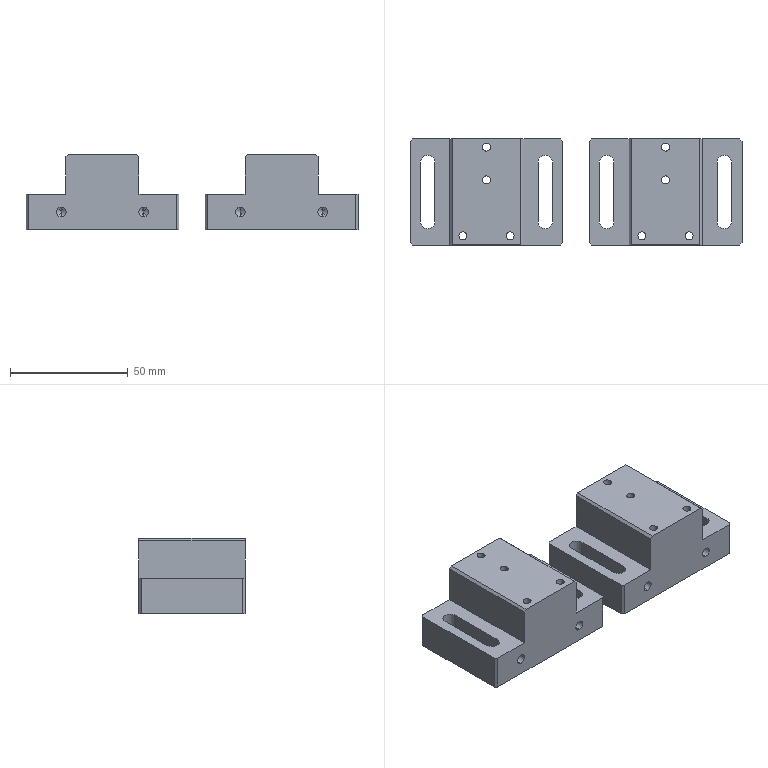Part | 2 solids | 104 faces | box 140.92 x 45 x 32 mm | volume 117955 mm3 | cylinder 48 | plane 48 | cone 8 | commonest cylinder face diameters 3.4 x16 6 x16 4.2 x8 6.2 x8